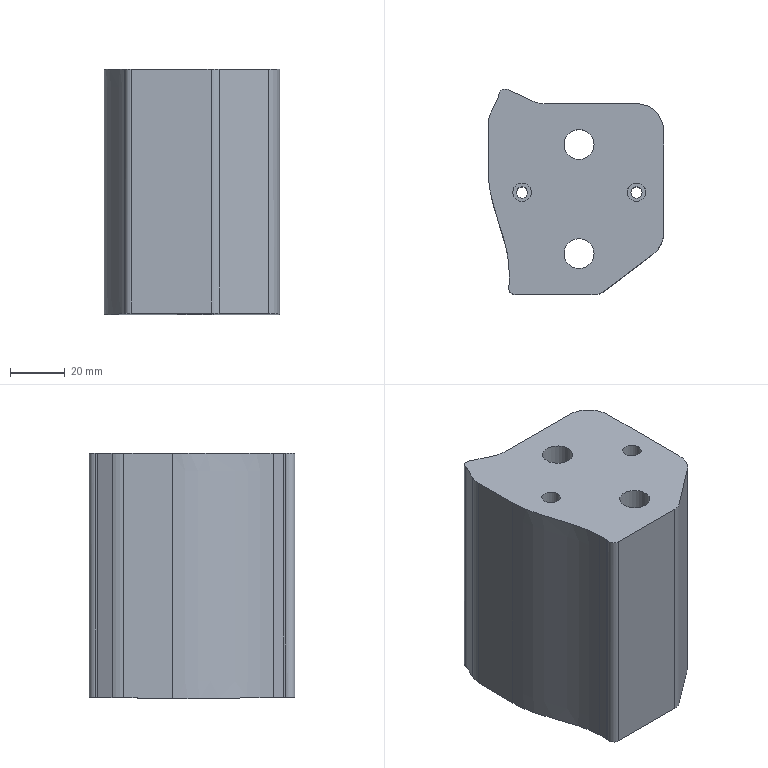Part | STEP file | gslz 2016.10.28-10_id2902_x_t | 1 solid | 34 faces | box 64.28 x 75.342 x 90 mm | volume 328224 mm3 | cylinder 17 | plane 14 | other 3 | commonest cylinder face diameters 5 x4 20 x3 4.1 x2 6.8 x2 11 x2 17 x2